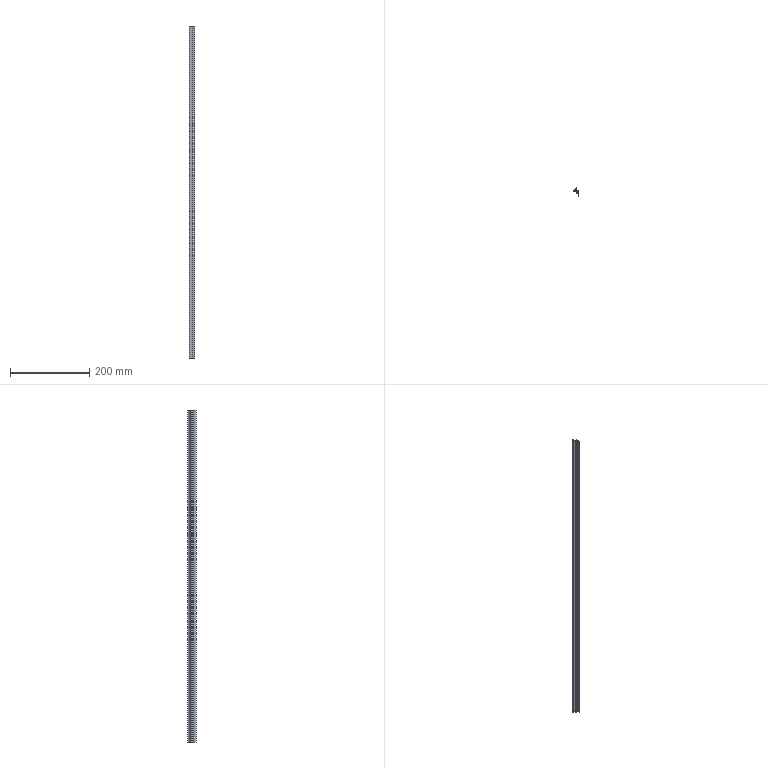Part | SolidWorks | features BaseBody 1, ICE 1, MoveFace 1 | 1 solid | 27 faces | box 14 x 20.3 x 840 mm | volume 42769 mm3 | plane 20 | cylinder 7 | commonest cylinder face diameters 0.387 x2 0.8 x2 0.4 x1 20 x1 22 x1
STEP:
#1=CARTESIAN_POINT('',(-5.304,-0.625,200.));
#2=VERTEX_POINT('',#1);
#3=CARTESIAN_POINT('',(-5.449,-0.8125,200.));
#4=VERTEX_POINT('',#3);
#5=CARTESIAN_POINT('',(-5.255,-0.8125,200.));
#6=DIRECTION('',(0.,0.,1.));
#7=DIRECTION('',(-1.,0.,0.));
#8=AXIS2_PLACEMENT_3D('',#5,#6,#7);
#9=CIRCLE('',#8,0.1937);
#10=EDGE_CURVE('',#2,#4,#9,.T.);
#11=ORIENTED_EDGE('',*,*,#10,.T.);
#12=CARTESIAN_POINT('',(-5.449,-0.8125,-640.));
#13=VERTEX_POINT('',#12);
#14=CARTESIAN_POINT('',(-5.449,-0.8125,230.));
#15=DIRECTION('',(0.,0.,-1.));
#16=VECTOR('',#15,1000.);
#17=LINE('',#14,#16);
#18=EDGE_CURVE('',#4,#13,#17,.T.);
#19=ORIENTED_EDGE('',*,*,#18,.T.);
#20=CARTESIAN_POINT('',(-5.304,-0.625,-640.));
#21=VERTEX_POINT('',#20);
#22=CARTESIAN_POINT('',(-5.255,-0.8125,-640.));
#23=DIRECTION('',(0.,0.,-1.));
#24=DIRECTION('',(1.,0.,0.));
#25=AXIS2_PLACEMENT_3D('',#22,#23,#24);
#26=CIRCLE('',#25,0.1937);
#27=EDGE_CURVE('',#13,#21,#26,.T.);
#28=ORIENTED_EDGE('',*,*,#27,.T.);
#29=CARTESIAN_POINT('',(-5.304,-0.625,230.));
#30=DIRECTION('',(0.,0.,-1.));
#31=VECTOR('',#30,1000.);
#32=LINE('',#29,#31);
#33=EDGE_CURVE('',#2,#21,#32,.T.);
#34=ORIENTED_EDGE('',*,*,#33,.F.);
#35=EDGE_LOOP('',(#11,#19,#28,#34));
#36=FACE_OUTER_BOUND('',#35,.T.);
#37=CARTESIAN_POINT('',(-5.255,-0.8125,230.));
#38=DIRECTION('',(0.,0.,-1.));
#39=DIRECTION('',(-1.,0.,0.));
#40=AXIS2_PLACEMENT_3D('',#37,#38,#39);
#41=CYLINDRICAL_SURFACE('',#40,0.1937);
#42=ADVANCED_FACE('',(#36),#41,.F.);
#43=CARTESIAN_POINT('',(5.,-1.,-640.));
#44=VERTEX_POINT('',#43);
#45=CARTESIAN_POINT('',(5.,-14.3,-640.));
#46=VERTEX_POINT('',#45);
#47=CARTESIAN_POINT('',(5.,29.623,-640.));
#48=DIRECTION('',(0.,-1.,0.));
#49=VECTOR('',#48,1000.);
#50=LINE('',#47,#49);
#51=EDGE_CURVE('',#44,#46,#50,.T.);
#52=ORIENTED_EDGE('',*,*,#51,.F.);
#53=CARTESIAN_POINT('',(5.,-1.,200.));
#54=VERTEX_POINT('',#53);
#55=CARTESIAN_POINT('',(5.,-1.,230.));
#56=DIRECTION('',(0.,0.,-1.));
#57=VECTOR('',#56,1000.);
#58=LINE('',#55,#57);
#59=EDGE_CURVE('',#54,#44,#58,.T.);
#60=ORIENTED_EDGE('',*,*,#59,.F.);
#61=CARTESIAN_POINT('',(5.,-14.3,200.));
#62=VERTEX_POINT('',#61);
#63=CARTESIAN_POINT('',(5.,-14.3,200.));
#64=DIRECTION('',(0.,1.,0.));
#65=VECTOR('',#64,1000.);
#66=LINE('',#63,#65);
#67=EDGE_CURVE('',#62,#54,#66,.T.);
#68=ORIENTED_EDGE('',*,*,#67,.F.);
#69=CARTESIAN_POINT('',(5.,-14.3,230.));
#70=DIRECTION('',(0.,0.,1.));
#71=VECTOR('',#70,1000.);
#72=LINE('',#69,#71);
#73=EDGE_CURVE('',#46,#62,#72,.T.);
#74=ORIENTED_EDGE('',*,*,#73,.F.);
#75=EDGE_LOOP('',(#52,#60,#68,#74));
#76=FACE_OUTER_BOUND('',#75,.T.);
#77=CARTESIAN_POINT('',(5.,-14.3,230.));
#78=DIRECTION('',(-1.,0.,0.));
#79=DIRECTION('',(0.,0.,1.));
#80=AXIS2_PLACEMENT_3D('',#77,#78,#79);
#81=PLANE('',#80);
#82=ADVANCED_FACE('',(#76),#81,.F.);
#83=CARTESIAN_POINT('',(-9.,-2.,-640.));
#84=VERTEX_POINT('',#83);
#85=CARTESIAN_POINT('',(-9.,-2.,200.));
#86=VERTEX_POINT('',#85);
#87=CARTESIAN_POINT('',(-9.,-2.,230.));
#88=DIRECTION('',(0.,0.,1.));
#89=VECTOR('',#88,1000.);
#90=LINE('',#87,#89);
#91=EDGE_CURVE('',#84,#86,#90,.T.);
#92=ORIENTED_EDGE('',*,*,#91,.F.);
#93=CARTESIAN_POINT('',(0.9,-2.,-640.));
#94=VERTEX_POINT('',#93);
#95=CARTESIAN_POINT('',(5.,-2.,-640.));
#96=DIRECTION('',(-1.,0.,0.));
#97=VECTOR('',#96,1000.);
#98=LINE('',#95,#97);
#99=EDGE_CURVE('',#94,#84,#98,.T.);
#100=ORIENTED_EDGE('',*,*,#99,.F.);
#101=CARTESIAN_POINT('',(0.9,-2.,200.));
#102=VERTEX_POINT('',#101);
#103=CARTESIAN_POINT('',(0.9,-2.,230.));
#104=DIRECTION('',(0.,0.,-1.));
#105=VECTOR('',#104,1000.);
#106=LINE('',#103,#105);
#107=EDGE_CURVE('',#102,#94,#106,.T.);
#108=ORIENTED_EDGE('',*,*,#107,.F.);
#109=CARTESIAN_POINT('',(5.,-2.,200.));
#110=DIRECTION('',(1.,0.,0.));
#111=VECTOR('',#110,1000.);
#112=LINE('',#109,#111);
#113=EDGE_CURVE('',#86,#102,#112,.T.);
#114=ORIENTED_EDGE('',*,*,#113,.F.);
#115=EDGE_LOOP('',(#92,#100,#108,#114));
#116=FACE_OUTER_BOUND('',#115,.T.);
#117=CARTESIAN_POINT('',(-9.,-2.,230.));
#118=DIRECTION('',(0.,1.,0.));
#119=DIRECTION('',(0.,0.,1.));
#120=AXIS2_PLACEMENT_3D('',#117,#118,#119);
#121=PLANE('',#120);
#122=ADVANCED_FACE('',(#116),#121,.F.);
#123=CARTESIAN_POINT('',(4.,-6.,200.));
#124=VERTEX_POINT('',#123);
#125=CARTESIAN_POINT('',(4.,-3.,200.));
#126=VERTEX_POINT('',#125);
#127=CARTESIAN_POINT('',(4.,29.623,200.));
#128=DIRECTION('',(0.,1.,0.));
#129=VECTOR('',#128,1000.);
#130=LINE('',#127,#129);
#131=EDGE_CURVE('',#124,#126,#130,.T.);
#132=ORIENTED_EDGE('',*,*,#131,.F.);
#133=CARTESIAN_POINT('',(1.,-6.,200.));
#134=VERTEX_POINT('',#133);
#135=CARTESIAN_POINT('',(5.,-6.,200.));
#136=DIRECTION('',(1.,0.,0.));
#137=VECTOR('',#136,1000.);
#138=LINE('',#135,#137);
#139=EDGE_CURVE('',#134,#124,#138,.T.);
#140=ORIENTED_EDGE('',*,*,#139,.F.);
#141=CARTESIAN_POINT('',(1.,-6.7,200.));
#142=VERTEX_POINT('',#141);
#143=CARTESIAN_POINT('',(1.,-6.,200.));
#144=DIRECTION('',(0.,-1.,0.));
#145=VECTOR('',#144,1000.);
#146=LINE('',#143,#145);
#147=EDGE_CURVE('',#134,#142,#146,.T.);
#148=ORIENTED_EDGE('',*,*,#147,.T.);
#149=CARTESIAN_POINT('',(-1.7,-6.7,200.));
#150=VERTEX_POINT('',#149);
#151=CARTESIAN_POINT('',(5.,-6.7,200.));
#152=DIRECTION('',(1.,0.,0.));
#153=VECTOR('',#152,1000.);
#154=LINE('',#151,#153);
#155=EDGE_CURVE('',#150,#142,#154,.T.);
#156=ORIENTED_EDGE('',*,*,#155,.F.);
#157=CARTESIAN_POINT('',(-1.7,-7.7,200.));
#158=VERTEX_POINT('',#157);
#159=CARTESIAN_POINT('',(-1.7,-6.7,200.));
#160=DIRECTION('',(0.,-1.,0.));
#161=VECTOR('',#160,1000.);
#162=LINE('',#159,#161);
#163=EDGE_CURVE('',#150,#158,#162,.T.);
#164=ORIENTED_EDGE('',*,*,#163,.T.);
#165=CARTESIAN_POINT('',(4.,-7.7,200.));
#166=VERTEX_POINT('',#165);
#167=CARTESIAN_POINT('',(5.,-7.7,200.));
#168=DIRECTION('',(-1.,0.,0.));
#169=VECTOR('',#168,1000.);
#170=LINE('',#167,#169);
#171=EDGE_CURVE('',#166,#158,#170,.T.);
#172=ORIENTED_EDGE('',*,*,#171,.F.);
#173=CARTESIAN_POINT('',(4.,-14.3,200.));
#174=VERTEX_POINT('',#173);
#175=CARTESIAN_POINT('',(4.,29.623,200.));
#176=DIRECTION('',(0.,1.,0.));
#177=VECTOR('',#176,1000.);
#178=LINE('',#175,#177);
#179=EDGE_CURVE('',#174,#166,#178,.T.);
#180=ORIENTED_EDGE('',*,*,#179,.F.);
#181=CARTESIAN_POINT('',(5.,-14.3,200.));
#182=DIRECTION('',(-1.,0.,0.));
#183=VECTOR('',#182,1000.);
#184=LINE('',#181,#183);
#185=EDGE_CURVE('',#62,#174,#184,.T.);
#186=ORIENTED_EDGE('',*,*,#185,.F.);
#187=ORIENTED_EDGE('',*,*,#67,.T.);
#188=CARTESIAN_POINT('',(-5.207,-1.,200.));
#189=VERTEX_POINT('',#188);
#190=CARTESIAN_POINT('',(5.,-1.,200.));
#191=DIRECTION('',(1.,0.,0.));
#192=VECTOR('',#191,1000.);
#193=LINE('',#190,#192);
#194=EDGE_CURVE('',#189,#54,#193,.T.);
#195=ORIENTED_EDGE('',*,*,#194,.F.);
#196=CARTESIAN_POINT('',(-5.255,-0.8125,200.));
#197=DIRECTION('',(0.,0.,1.));
#198=DIRECTION('',(-1.,0.,0.));
#199=AXIS2_PLACEMENT_3D('',#196,#197,#198);
#200=CIRCLE('',#199,0.1937);
#201=EDGE_CURVE('',#4,#189,#200,.T.);
#202=ORIENTED_EDGE('',*,*,#201,.F.);
#203=ORIENTED_EDGE('',*,*,#10,.F.);
#204=CARTESIAN_POINT('',(-1.368,3.063,200.));
#205=VERTEX_POINT('',#204);
#206=CARTESIAN_POINT('',(-10.628,9.,200.));
#207=DIRECTION('',(0.,0.,1.));
#208=DIRECTION('',(-1.,0.,0.));
#209=AXIS2_PLACEMENT_3D('',#206,#207,#208);
#210=CIRCLE('',#209,11.);
#211=EDGE_CURVE('',#2,#205,#210,.T.);
#212=ORIENTED_EDGE('',*,*,#211,.T.);
#213=CARTESIAN_POINT('',(-1.,2.955,200.));
#214=VERTEX_POINT('',#213);
#215=CARTESIAN_POINT('',(-1.2,2.955,200.));
#216=DIRECTION('',(0.,0.,1.));
#217=DIRECTION('',(-1.,0.,0.));
#218=AXIS2_PLACEMENT_3D('',#215,#216,#217);
#219=CIRCLE('',#218,0.2);
#220=EDGE_CURVE('',#214,#205,#219,.T.);
#221=ORIENTED_EDGE('',*,*,#220,.F.);
#222=CARTESIAN_POINT('',(-1.,1.5,200.));
#223=VERTEX_POINT('',#222);
#224=CARTESIAN_POINT('',(-1.,2.955,200.));
#225=DIRECTION('',(0.,1.,0.));
#226=VECTOR('',#225,1000.);
#227=LINE('',#224,#226);
#228=EDGE_CURVE('',#223,#214,#227,.T.);
#229=ORIENTED_EDGE('',*,*,#228,.F.);
#230=CARTESIAN_POINT('',(0.,1.5,200.));
#231=VERTEX_POINT('',#230);
#232=CARTESIAN_POINT('',(-1.,1.5,200.));
#233=DIRECTION('',(-1.,0.,0.));
#234=VECTOR('',#233,1000.);
#235=LINE('',#232,#234);
#236=EDGE_CURVE('',#231,#223,#235,.T.);
#237=ORIENTED_EDGE('',*,*,#236,.F.);
#238=CARTESIAN_POINT('',(0.,6.,200.));
#239=VERTEX_POINT('',#238);
#240=CARTESIAN_POINT('',(0.,1.5,200.));
#241=DIRECTION('',(0.,-1.,0.));
#242=VECTOR('',#241,1000.);
#243=LINE('',#240,#242);
#244=EDGE_CURVE('',#239,#231,#243,.T.);
#245=ORIENTED_EDGE('',*,*,#244,.F.);
#246=CARTESIAN_POINT('',(-0.8,6.,200.));
#247=VERTEX_POINT('',#246);
#248=CARTESIAN_POINT('',(0.,6.,200.));
#249=DIRECTION('',(1.,0.,0.));
#250=VECTOR('',#249,1000.);
#251=LINE('',#248,#250);
#252=EDGE_CURVE('',#247,#239,#251,.T.);
#253=ORIENTED_EDGE('',*,*,#252,.F.);
#254=CARTESIAN_POINT('',(-1.178,5.731,200.));
#255=VERTEX_POINT('',#254);
#256=CARTESIAN_POINT('',(-0.8,5.6,200.));
#257=DIRECTION('',(0.,0.,1.));
#258=DIRECTION('',(-1.,0.,0.));
#259=AXIS2_PLACEMENT_3D('',#256,#257,#258);
#260=CIRCLE('',#259,0.4);
#261=EDGE_CURVE('',#247,#255,#260,.T.);
#262=ORIENTED_EDGE('',*,*,#261,.T.);
#263=CARTESIAN_POINT('',(-8.678,-0.8077,200.));
#264=VERTEX_POINT('',#263);
#265=CARTESIAN_POINT('',(-10.628,9.,200.));
#266=DIRECTION('',(0.,0.,1.));
#267=DIRECTION('',(-1.,0.,0.));
#268=AXIS2_PLACEMENT_3D('',#265,#266,#267);
#269=CIRCLE('',#268,10.);
#270=EDGE_CURVE('',#264,#255,#269,.T.);
#271=ORIENTED_EDGE('',*,*,#270,.F.);
#272=CARTESIAN_POINT('',(-9.,-1.2,200.));
#273=VERTEX_POINT('',#272);
#274=CARTESIAN_POINT('',(-8.6,-1.2,200.));
#275=DIRECTION('',(0.,0.,1.));
#276=DIRECTION('',(-1.,0.,0.));
#277=AXIS2_PLACEMENT_3D('',#274,#275,#276);
#278=CIRCLE('',#277,0.4);
#279=EDGE_CURVE('',#264,#273,#278,.T.);
#280=ORIENTED_EDGE('',*,*,#279,.T.);
#281=CARTESIAN_POINT('',(-9.,8.,200.));
#282=DIRECTION('',(0.,-1.,0.));
#283=VECTOR('',#282,1000.);
#284=LINE('',#281,#283);
#285=EDGE_CURVE('',#273,#86,#284,.T.);
#286=ORIENTED_EDGE('',*,*,#285,.T.);
#287=ORIENTED_EDGE('',*,*,#113,.T.);
#288=CARTESIAN_POINT('',(0.9,-3.,200.));
#289=VERTEX_POINT('',#288);
#290=CARTESIAN_POINT('',(0.9,29.623,200.));
#291=DIRECTION('',(0.,1.,0.));
#292=VECTOR('',#291,1000.);
#293=LINE('',#290,#292);
#294=EDGE_CURVE('',#289,#102,#293,.T.);
#295=ORIENTED_EDGE('',*,*,#294,.F.);
#296=CARTESIAN_POINT('',(5.,-3.,200.));
#297=DIRECTION('',(-1.,0.,0.));
#298=VECTOR('',#297,1000.);
#299=LINE('',#296,#298);
#300=EDGE_CURVE('',#126,#289,#299,.T.);
#301=ORIENTED_EDGE('',*,*,#300,.F.);
#302=EDGE_LOOP('',(#132,#140,#148,#156,#164,#172,#180,#186,#187,#195,#202,#203,#212,#221,#229,#237,#245,#253,#262,#271,#280,#286,#287,#295,#301));
#303=FACE_OUTER_BOUND('',#302,.T.);
#304=CARTESIAN_POINT('',(5.,29.623,200.));
#305=DIRECTION('',(0.,0.,-1.));
#306=DIRECTION('',(-1.,0.,0.));
#307=AXIS2_PLACEMENT_3D('',#304,#305,#306);
#308=PLANE('',#307);
#309=ADVANCED_FACE('',(#303),#308,.F.);
#310=ORIENTED_EDGE('',*,*,#185,.T.);
#311=CARTESIAN_POINT('',(4.,-14.3,-640.));
#312=VERTEX_POINT('',#311);
#313=CARTESIAN_POINT('',(4.,-14.3,230.));
#314=DIRECTION('',(0.,0.,1.));
#315=VECTOR('',#314,1000.);
#316=LINE('',#313,#315);
#317=EDGE_CURVE('',#312,#174,#316,.T.);
#318=ORIENTED_EDGE('',*,*,#317,.F.);
#319=CARTESIAN_POINT('',(5.,-14.3,-640.));
#320=DIRECTION('',(-1.,0.,0.));
#321=VECTOR('',#320,1000.);
#322=LINE('',#319,#321);
#323=EDGE_CURVE('',#46,#312,#322,.T.);
#324=ORIENTED_EDGE('',*,*,#323,.F.);
#325=ORIENTED_EDGE('',*,*,#73,.T.);
#326=EDGE_LOOP('',(#310,#318,#324,#325));
#327=FACE_OUTER_BOUND('',#326,.T.);
#328=CARTESIAN_POINT('',(4.,-14.3,230.));
#329=DIRECTION('',(0.,1.,0.));
#330=DIRECTION('',(0.,0.,1.));
#331=AXIS2_PLACEMENT_3D('',#328,#329,#330);
#332=PLANE('',#331);
#333=ADVANCED_FACE('',(#327),#332,.F.);
#334=ORIENTED_EDGE('',*,*,#51,.T.);
#335=ORIENTED_EDGE('',*,*,#323,.T.);
#336=CARTESIAN_POINT('',(4.,-7.7,-640.));
#337=VERTEX_POINT('',#336);
#338=CARTESIAN_POINT('',(4.,-7.7,-640.));
#339=DIRECTION('',(0.,-1.,0.));
#340=VECTOR('',#339,1000.);
#341=LINE('',#338,#340);
#342=EDGE_CURVE('',#337,#312,#341,.T.);
#343=ORIENTED_EDGE('',*,*,#342,.F.);
#344=CARTESIAN_POINT('',(-1.7,-7.7,-640.));
#345=VERTEX_POINT('',#344);
#346=CARTESIAN_POINT('',(-1.7,-7.7,-640.));
#347=DIRECTION('',(1.,0.,0.));
#348=VECTOR('',#347,1000.);
#349=LINE('',#346,#348);
#350=EDGE_CURVE('',#345,#337,#349,.T.);
#351=ORIENTED_EDGE('',*,*,#350,.F.);
#352=CARTESIAN_POINT('',(-1.7,-6.7,-640.));
#353=VERTEX_POINT('',#352);
#354=CARTESIAN_POINT('',(-1.7,29.623,-640.));
#355=DIRECTION('',(0.,1.,0.));
#356=VECTOR('',#355,1000.);
#357=LINE('',#354,#356);
#358=EDGE_CURVE('',#345,#353,#357,.T.);
#359=ORIENTED_EDGE('',*,*,#358,.T.);
#360=CARTESIAN_POINT('',(1.,-6.7,-640.));
#361=VERTEX_POINT('',#360);
#362=CARTESIAN_POINT('',(1.,-6.7,-640.));
#363=DIRECTION('',(-1.,0.,0.));
#364=VECTOR('',#363,1000.);
#365=LINE('',#362,#364);
#366=EDGE_CURVE('',#361,#353,#365,.T.);
#367=ORIENTED_EDGE('',*,*,#366,.F.);
#368=CARTESIAN_POINT('',(1.,-6.,-640.));
#369=VERTEX_POINT('',#368);
#370=CARTESIAN_POINT('',(1.,29.623,-640.));
#371=DIRECTION('',(0.,1.,0.));
#372=VECTOR('',#371,1000.);
#373=LINE('',#370,#372);
#374=EDGE_CURVE('',#361,#369,#373,.T.);
#375=ORIENTED_EDGE('',*,*,#374,.T.);
#376=CARTESIAN_POINT('',(4.,-6.,-640.));
#377=VERTEX_POINT('',#376);
#378=CARTESIAN_POINT('',(4.,-6.,-640.));
#379=DIRECTION('',(-1.,0.,0.));
#380=VECTOR('',#379,1000.);
#381=LINE('',#378,#380);
#382=EDGE_CURVE('',#377,#369,#381,.T.);
#383=ORIENTED_EDGE('',*,*,#382,.F.);
#384=CARTESIAN_POINT('',(4.,-3.,-640.));
#385=VERTEX_POINT('',#384);
#386=CARTESIAN_POINT('',(4.,-3.,-640.));
#387=DIRECTION('',(0.,-1.,0.));
#388=VECTOR('',#387,1000.);
#389=LINE('',#386,#388);
#390=EDGE_CURVE('',#385,#377,#389,.T.);
#391=ORIENTED_EDGE('',*,*,#390,.F.);
#392=CARTESIAN_POINT('',(0.9,-3.,-640.));
#393=VERTEX_POINT('',#392);
#394=CARTESIAN_POINT('',(0.9,-3.,-640.));
#395=DIRECTION('',(1.,0.,0.));
#396=VECTOR('',#395,1000.);
#397=LINE('',#394,#396);
#398=EDGE_CURVE('',#393,#385,#397,.T.);
#399=ORIENTED_EDGE('',*,*,#398,.F.);
#400=CARTESIAN_POINT('',(0.9,-2.,-640.));
#401=DIRECTION('',(0.,-1.,0.));
#402=VECTOR('',#401,1000.);
#403=LINE('',#400,#402);
#404=EDGE_CURVE('',#94,#393,#403,.T.);
#405=ORIENTED_EDGE('',*,*,#404,.F.);
#406=ORIENTED_EDGE('',*,*,#99,.T.);
#407=CARTESIAN_POINT('',(-9.,-1.2,-640.));
#408=VERTEX_POINT('',#407);
#409=CARTESIAN_POINT('',(-9.,-1.2,-640.));
#410=DIRECTION('',(0.,-1.,0.));
#411=VECTOR('',#410,1000.);
#412=LINE('',#409,#411);
#413=EDGE_CURVE('',#408,#84,#412,.T.);
#414=ORIENTED_EDGE('',*,*,#413,.F.);
#415=CARTESIAN_POINT('',(-8.678,-0.8077,-640.));
#416=VERTEX_POINT('',#415);
#417=CARTESIAN_POINT('',(-8.6,-1.2,-640.));
#418=DIRECTION('',(0.,0.,-1.));
#419=DIRECTION('',(1.,0.,0.));
#420=AXIS2_PLACEMENT_3D('',#417,#418,#419);
#421=CIRCLE('',#420,0.4);
#422=EDGE_CURVE('',#408,#416,#421,.T.);
#423=ORIENTED_EDGE('',*,*,#422,.T.);
#424=CARTESIAN_POINT('',(-1.178,5.731,-640.));
#425=VERTEX_POINT('',#424);
#426=CARTESIAN_POINT('',(-10.628,9.,-640.));
#427=DIRECTION('',(0.,0.,-1.));
#428=DIRECTION('',(1.,0.,0.));
#429=AXIS2_PLACEMENT_3D('',#426,#427,#428);
#430=CIRCLE('',#429,10.);
#431=EDGE_CURVE('',#425,#416,#430,.T.);
#432=ORIENTED_EDGE('',*,*,#431,.F.);
#433=CARTESIAN_POINT('',(-0.8,6.,-640.));
#434=VERTEX_POINT('',#433);
#435=CARTESIAN_POINT('',(-0.8,5.6,-640.));
#436=DIRECTION('',(0.,0.,-1.));
#437=DIRECTION('',(1.,0.,0.));
#438=AXIS2_PLACEMENT_3D('',#435,#436,#437);
#439=CIRCLE('',#438,0.4);
#440=EDGE_CURVE('',#425,#434,#439,.T.);
#441=ORIENTED_EDGE('',*,*,#440,.T.);
#442=CARTESIAN_POINT('',(0.,6.,-640.));
#443=VERTEX_POINT('',#442);
#444=CARTESIAN_POINT('',(0.,6.,-640.));
#445=DIRECTION('',(-1.,0.,0.));
#446=VECTOR('',#445,1000.);
#447=LINE('',#444,#446);
#448=EDGE_CURVE('',#443,#434,#447,.T.);
#449=ORIENTED_EDGE('',*,*,#448,.F.);
#450=CARTESIAN_POINT('',(0.,1.5,-640.));
#451=VERTEX_POINT('',#450);
#452=CARTESIAN_POINT('',(0.,1.5,-640.));
#453=DIRECTION('',(0.,1.,0.));
#454=VECTOR('',#453,1000.);
#455=LINE('',#452,#454);
#456=EDGE_CURVE('',#451,#443,#455,.T.);
#457=ORIENTED_EDGE('',*,*,#456,.F.);
#458=CARTESIAN_POINT('',(-1.,1.5,-640.));
#459=VERTEX_POINT('',#458);
#460=CARTESIAN_POINT('',(-1.,1.5,-640.));
#461=DIRECTION('',(1.,0.,0.));
#462=VECTOR('',#461,1000.);
#463=LINE('',#460,#462);
#464=EDGE_CURVE('',#459,#451,#463,.T.);
#465=ORIENTED_EDGE('',*,*,#464,.F.);
#466=CARTESIAN_POINT('',(-1.,2.955,-640.));
#467=VERTEX_POINT('',#466);
#468=CARTESIAN_POINT('',(-1.,2.955,-640.));
#469=DIRECTION('',(0.,-1.,0.));
#470=VECTOR('',#469,1000.);
#471=LINE('',#468,#470);
#472=EDGE_CURVE('',#467,#459,#471,.T.);
#473=ORIENTED_EDGE('',*,*,#472,.F.);
#474=CARTESIAN_POINT('',(-1.368,3.063,-640.));
#475=VERTEX_POINT('',#474);
#476=CARTESIAN_POINT('',(-1.2,2.955,-640.));
#477=DIRECTION('',(0.,0.,-1.));
#478=DIRECTION('',(1.,0.,0.));
#479=AXIS2_PLACEMENT_3D('',#476,#477,#478);
#480=CIRCLE('',#479,0.2);
#481=EDGE_CURVE('',#475,#467,#480,.T.);
#482=ORIENTED_EDGE('',*,*,#481,.F.);
#483=CARTESIAN_POINT('',(-10.628,9.,-640.));
#484=DIRECTION('',(0.,0.,-1.));
#485=DIRECTION('',(1.,0.,0.));
#486=AXIS2_PLACEMENT_3D('',#483,#484,#485);
#487=CIRCLE('',#486,11.);
#488=EDGE_CURVE('',#475,#21,#487,.T.);
#489=ORIENTED_EDGE('',*,*,#488,.T.);
#490=ORIENTED_EDGE('',*,*,#27,.F.);
#491=CARTESIAN_POINT('',(-5.207,-1.,-640.));
#492=VERTEX_POINT('',#491);
#493=CARTESIAN_POINT('',(-5.255,-0.8125,-640.));
#494=DIRECTION('',(0.,0.,-1.));
#495=DIRECTION('',(1.,0.,0.));
#496=AXIS2_PLACEMENT_3D('',#493,#494,#495);
#497=CIRCLE('',#496,0.1937);
#498=EDGE_CURVE('',#492,#13,#497,.T.);
#499=ORIENTED_EDGE('',*,*,#498,.F.);
#500=CARTESIAN_POINT('',(5.,-1.,-640.));
#501=DIRECTION('',(-1.,0.,0.));
#502=VECTOR('',#501,1000.);
#503=LINE('',#500,#502);
#504=EDGE_CURVE('',#44,#492,#503,.T.);
#505=ORIENTED_EDGE('',*,*,#504,.F.);
#506=EDGE_LOOP('',(#334,#335,#343,#351,#359,#367,#375,#383,#391,#399,#405,#406,#414,#423,#432,#441,#449,#457,#465,#473,#482,#489,#490,#499,#505));
#507=FACE_OUTER_BOUND('',#506,.T.);
#508=CARTESIAN_POINT('',(5.,29.623,-640.));
#509=DIRECTION('',(0.,0.,1.));
#510=DIRECTION('',(1.,0.,0.));
#511=AXIS2_PLACEMENT_3D('',#508,#509,#510);
#512=PLANE('',#511);
#513=ADVANCED_FACE('',(#507),#512,.F.);
#514=ORIENTED_EDGE('',*,*,#59,.T.);
#515=ORIENTED_EDGE('',*,*,#504,.T.);
#516=CARTESIAN_POINT('',(-5.207,-1.,230.));
#517=DIRECTION('',(0.,0.,-1.));
#518=VECTOR('',#517,1000.);
#519=LINE('',#516,#518);
#520=EDGE_CURVE('',#189,#492,#519,.T.);
#521=ORIENTED_EDGE('',*,*,#520,.F.);
#522=ORIENTED_EDGE('',*,*,#194,.T.);
#523=EDGE_LOOP('',(#514,#515,#521,#522));
#524=FACE_OUTER_BOUND('',#523,.T.);
#525=CARTESIAN_POINT('',(5.,-1.,230.));
#526=DIRECTION('',(0.,-1.,0.));
#527=DIRECTION('',(0.,0.,-1.));
#528=AXIS2_PLACEMENT_3D('',#525,#526,#527);
#529=PLANE('',#528);
#530=ADVANCED_FACE('',(#524),#529,.F.);
#531=CARTESIAN_POINT('',(-9.,-1.2,230.));
#532=DIRECTION('',(0.,0.,1.));
#533=VECTOR('',#532,1000.);
#534=LINE('',#531,#533);
#535=EDGE_CURVE('',#408,#273,#534,.T.);
#536=ORIENTED_EDGE('',*,*,#535,.F.);
#537=ORIENTED_EDGE('',*,*,#413,.T.);
#538=ORIENTED_EDGE('',*,*,#91,.T.);
#539=ORIENTED_EDGE('',*,*,#285,.F.);
#540=EDGE_LOOP('',(#536,#537,#538,#539));
#541=FACE_OUTER_BOUND('',#540,.T.);
#542=CARTESIAN_POINT('',(-9.,-1.2,230.));
#543=DIRECTION('',(1.,0.,0.));
#544=DIRECTION('',(0.,0.,-1.));
#545=AXIS2_PLACEMENT_3D('',#542,#543,#544);
#546=PLANE('',#545);
#547=ADVANCED_FACE('',(#541),#546,.F.);
#548=ORIENTED_EDGE('',*,*,#294,.T.);
#549=ORIENTED_EDGE('',*,*,#107,.T.);
#550=ORIENTED_EDGE('',*,*,#404,.T.);
#551=CARTESIAN_POINT('',(0.9,-3.,230.));
#552=DIRECTION('',(0.,0.,-1.));
#553=VECTOR('',#552,1000.);
#554=LINE('',#551,#553);
#555=EDGE_CURVE('',#289,#393,#554,.T.);
#556=ORIENTED_EDGE('',*,*,#555,.F.);
#557=EDGE_LOOP('',(#548,#549,#550,#556));
#558=FACE_OUTER_BOUND('',#557,.T.);
#559=CARTESIAN_POINT('',(0.9,-2.,230.));
#560=DIRECTION('',(1.,0.,0.));
#561=DIRECTION('',(0.,0.,-1.));
#562=AXIS2_PLACEMENT_3D('',#559,#560,#561);
#563=PLANE('',#562);
#564=ADVANCED_FACE('',(#558),#563,.F.);
#565=ORIENTED_EDGE('',*,*,#300,.T.);
#566=ORIENTED_EDGE('',*,*,#555,.T.);
#567=ORIENTED_EDGE('',*,*,#398,.T.);
#568=CARTESIAN_POINT('',(4.,-3.,230.));
#569=DIRECTION('',(0.,0.,-1.));
#570=VECTOR('',#569,1000.);
#571=LINE('',#568,#570);
#572=EDGE_CURVE('',#126,#385,#571,.T.);
#573=ORIENTED_EDGE('',*,*,#572,.F.);
#574=EDGE_LOOP('',(#565,#566,#567,#573));
#575=FACE_OUTER_BOUND('',#574,.T.);
#576=CARTESIAN_POINT('',(0.9,-3.,230.));
#577=DIRECTION('',(0.,1.,0.));
#578=DIRECTION('',(0.,0.,1.));
#579=AXIS2_PLACEMENT_3D('',#576,#577,#578);
#580=PLANE('',#579);
#581=ADVANCED_FACE('',(#575),#580,.F.);
#582=ORIENTED_EDGE('',*,*,#131,.T.);
#583=ORIENTED_EDGE('',*,*,#572,.T.);
#584=ORIENTED_EDGE('',*,*,#390,.T.);
#585=CARTESIAN_POINT('',(4.,-6.,230.));
#586=DIRECTION('',(0.,0.,-1.));
#587=VECTOR('',#586,1000.);
#588=LINE('',#585,#587);
#589=EDGE_CURVE('',#124,#377,#588,.T.);
#590=ORIENTED_EDGE('',*,*,#589,.F.);
#591=EDGE_LOOP('',(#582,#583,#584,#590));
#592=FACE_OUTER_BOUND('',#591,.T.);
#593=CARTESIAN_POINT('',(4.,-3.,230.));
#594=DIRECTION('',(1.,0.,0.));
#595=DIRECTION('',(0.,0.,-1.));
#596=AXIS2_PLACEMENT_3D('',#593,#594,#595);
#597=PLANE('',#596);
#598=ADVANCED_FACE('',(#592),#597,.F.);
#599=ORIENTED_EDGE('',*,*,#139,.T.);
#600=ORIENTED_EDGE('',*,*,#589,.T.);
#601=ORIENTED_EDGE('',*,*,#382,.T.);
#602=CARTESIAN_POINT('',(1.,-6.,230.));
#603=DIRECTION('',(0.,0.,-1.));
#604=VECTOR('',#603,1000.);
#605=LINE('',#602,#604);
#606=EDGE_CURVE('',#134,#369,#605,.T.);
#607=ORIENTED_EDGE('',*,*,#606,.F.);
#608=EDGE_LOOP('',(#599,#600,#601,#607));
#609=FACE_OUTER_BOUND('',#608,.T.);
#610=CARTESIAN_POINT('',(4.,-6.,230.));
#611=DIRECTION('',(0.,-1.,0.));
#612=DIRECTION('',(0.,0.,-1.));
#613=AXIS2_PLACEMENT_3D('',#610,#611,#612);
#614=PLANE('',#613);
#615=ADVANCED_FACE('',(#609),#614,.F.);
#616=ORIENTED_EDGE('',*,*,#155,.T.);
#617=CARTESIAN_POINT('',(1.,-6.7,230.));
#618=DIRECTION('',(0.,0.,1.));
#619=VECTOR('',#618,1000.);
#620=LINE('',#617,#619);
#621=EDGE_CURVE('',#361,#142,#620,.T.);
#622=ORIENTED_EDGE('',*,*,#621,.F.);
#623=ORIENTED_EDGE('',*,*,#366,.T.);
#624=CARTESIAN_POINT('',(-1.7,-6.7,230.));
#625=DIRECTION('',(0.,0.,-1.));
#626=VECTOR('',#625,1000.);
#627=LINE('',#624,#626);
#628=EDGE_CURVE('',#150,#353,#627,.T.);
#629=ORIENTED_EDGE('',*,*,#628,.F.);
#630=EDGE_LOOP('',(#616,#622,#623,#629));
#631=FACE_OUTER_BOUND('',#630,.T.);
#632=CARTESIAN_POINT('',(1.,-6.7,230.));
#633=DIRECTION('',(0.,-1.,0.));
#634=DIRECTION('',(0.,0.,-1.));
#635=AXIS2_PLACEMENT_3D('',#632,#633,#634);
#636=PLANE('',#635);
#637=ADVANCED_FACE('',(#631),#636,.F.);
#638=ORIENTED_EDGE('',*,*,#171,.T.);
#639=CARTESIAN_POINT('',(-1.7,-7.7,230.));
#640=DIRECTION('',(0.,0.,1.));
#641=VECTOR('',#640,1000.);
#642=LINE('',#639,#641);
#643=EDGE_CURVE('',#345,#158,#642,.T.);
#644=ORIENTED_EDGE('',*,*,#643,.F.);
#645=ORIENTED_EDGE('',*,*,#350,.T.);
#646=CARTESIAN_POINT('',(4.,-7.7,230.));
#647=DIRECTION('',(0.,0.,-1.));
#648=VECTOR('',#647,1000.);
#649=LINE('',#646,#648);
#650=EDGE_CURVE('',#166,#337,#649,.T.);
#651=ORIENTED_EDGE('',*,*,#650,.F.);
#652=EDGE_LOOP('',(#638,#644,#645,#651));
#653=FACE_OUTER_BOUND('',#652,.T.);
#654=CARTESIAN_POINT('',(-1.7,-7.7,230.));
#655=DIRECTION('',(0.,1.,0.));
#656=DIRECTION('',(0.,0.,1.));
#657=AXIS2_PLACEMENT_3D('',#654,#655,#656);
#658=PLANE('',#657);
#659=ADVANCED_FACE('',(#653),#658,.F.);
#660=ORIENTED_EDGE('',*,*,#179,.T.);
#661=ORIENTED_EDGE('',*,*,#650,.T.);
#662=ORIENTED_EDGE('',*,*,#342,.T.);
#663=ORIENTED_EDGE('',*,*,#317,.T.);
#664=EDGE_LOOP('',(#660,#661,#662,#663));
#665=FACE_OUTER_BOUND('',#664,.T.);
#666=CARTESIAN_POINT('',(4.,-7.7,230.));
#667=DIRECTION('',(1.,0.,0.));
#668=DIRECTION('',(0.,0.,-1.));
#669=AXIS2_PLACEMENT_3D('',#666,#667,#668);
#670=PLANE('',#669);
#671=ADVANCED_FACE('',(#665),#670,.F.);
#672=ORIENTED_EDGE('',*,*,#18,.F.);
#673=ORIENTED_EDGE('',*,*,#201,.T.);
#674=ORIENTED_EDGE('',*,*,#520,.T.);
#675=ORIENTED_EDGE('',*,*,#498,.T.);
#676=EDGE_LOOP('',(#672,#673,#674,#675));
#677=FACE_OUTER_BOUND('',#676,.T.);
#678=CARTESIAN_POINT('',(-5.255,-0.8125,230.));
#679=DIRECTION('',(0.,0.,-1.));
#680=DIRECTION('',(-1.,0.,0.));
#681=AXIS2_PLACEMENT_3D('',#678,#679,#680);
#682=CYLINDRICAL_SURFACE('',#681,0.1937);
#683=ADVANCED_FACE('',(#677),#682,.F.);
#684=CARTESIAN_POINT('',(-1.,2.955,230.));
#685=DIRECTION('',(0.,0.,1.));
#686=VECTOR('',#685,1000.);
#687=LINE('',#684,#686);
#688=EDGE_CURVE('',#467,#214,#687,.T.);
#689=ORIENTED_EDGE('',*,*,#688,.F.);
#690=ORIENTED_EDGE('',*,*,#472,.T.);
#691=CARTESIAN_POINT('',(-1.,1.5,230.));
#692=DIRECTION('',(0.,0.,-1.));
#693=VECTOR('',#692,1000.);
#694=LINE('',#691,#693);
#695=EDGE_CURVE('',#223,#459,#694,.T.);
#696=ORIENTED_EDGE('',*,*,#695,.F.);
#697=ORIENTED_EDGE('',*,*,#228,.T.);
#698=EDGE_LOOP('',(#689,#690,#696,#697));
#699=FACE_OUTER_BOUND('',#698,.T.);
#700=CARTESIAN_POINT('',(-1.,2.955,230.));
#701=DIRECTION('',(1.,0.,0.));
#702=DIRECTION('',(0.,0.,-1.));
#703=AXIS2_PLACEMENT_3D('',#700,#701,#702);
#704=PLANE('',#703);
#705=ADVANCED_FACE('',(#699),#704,.F.);
#706=ORIENTED_EDGE('',*,*,#488,.F.);
#707=CARTESIAN_POINT('',(-1.368,3.063,230.));
#708=DIRECTION('',(0.,0.,1.));
#709=VECTOR('',#708,1000.);
#710=LINE('',#707,#709);
#711=EDGE_CURVE('',#475,#205,#710,.T.);
#712=ORIENTED_EDGE('',*,*,#711,.T.);
#713=ORIENTED_EDGE('',*,*,#211,.F.);
#714=ORIENTED_EDGE('',*,*,#33,.T.);
#715=EDGE_LOOP('',(#706,#712,#713,#714));
#716=FACE_OUTER_BOUND('',#715,.T.);
#717=CARTESIAN_POINT('',(-10.628,9.,230.));
#718=DIRECTION('',(0.,0.,-1.));
#719=DIRECTION('',(-1.,0.,0.));
#720=AXIS2_PLACEMENT_3D('',#717,#718,#719);
#721=CYLINDRICAL_SURFACE('',#720,11.);
#722=ADVANCED_FACE('',(#716),#721,.T.);
#723=CARTESIAN_POINT('',(-1.178,5.731,230.));
#724=DIRECTION('',(0.,0.,1.));
#725=VECTOR('',#724,1000.);
#726=LINE('',#723,#725);
#727=EDGE_CURVE('',#425,#255,#726,.T.);
#728=ORIENTED_EDGE('',*,*,#727,.F.);
#729=ORIENTED_EDGE('',*,*,#431,.T.);
#730=CARTESIAN_POINT('',(-8.678,-0.8077,230.));
#731=DIRECTION('',(0.,0.,-1.));
#732=VECTOR('',#731,1000.);
#733=LINE('',#730,#732);
#734=EDGE_CURVE('',#264,#416,#733,.T.);
#735=ORIENTED_EDGE('',*,*,#734,.F.);
#736=ORIENTED_EDGE('',*,*,#270,.T.);
#737=EDGE_LOOP('',(#728,#729,#735,#736));
#738=FACE_OUTER_BOUND('',#737,.T.);
#739=CARTESIAN_POINT('',(-10.628,9.,230.));
#740=DIRECTION('',(0.,0.,-1.));
#741=DIRECTION('',(-1.,0.,0.));
#742=AXIS2_PLACEMENT_3D('',#739,#740,#741);
#743=CYLINDRICAL_SURFACE('',#742,10.);
#744=ADVANCED_FACE('',(#738),#743,.F.);
#745=CARTESIAN_POINT('',(0.,1.5,230.));
#746=DIRECTION('',(0.,0.,1.));
#747=VECTOR('',#746,1000.);
#748=LINE('',#745,#747);
#749=EDGE_CURVE('',#451,#231,#748,.T.);
#750=ORIENTED_EDGE('',*,*,#749,.F.);
#751=ORIENTED_EDGE('',*,*,#456,.T.);
#752=CARTESIAN_POINT('',(0.,6.,230.));
#753=DIRECTION('',(0.,0.,-1.));
#754=VECTOR('',#753,1000.);
#755=LINE('',#752,#754);
#756=EDGE_CURVE('',#239,#443,#755,.T.);
#757=ORIENTED_EDGE('',*,*,#756,.F.);
#758=ORIENTED_EDGE('',*,*,#244,.T.);
#759=EDGE_LOOP('',(#750,#751,#757,#758));
#760=FACE_OUTER_BOUND('',#759,.T.);
#761=CARTESIAN_POINT('',(0.,1.5,230.));
#762=DIRECTION('',(-1.,0.,0.));
#763=DIRECTION('',(0.,0.,1.));
#764=AXIS2_PLACEMENT_3D('',#761,#762,#763);
#765=PLANE('',#764);
#766=ADVANCED_FACE('',(#760),#765,.F.);
#767=ORIENTED_EDGE('',*,*,#422,.F.);
#768=ORIENTED_EDGE('',*,*,#535,.T.);
#769=ORIENTED_EDGE('',*,*,#279,.F.);
#770=ORIENTED_EDGE('',*,*,#734,.T.);
#771=EDGE_LOOP('',(#767,#768,#769,#770));
#772=FACE_OUTER_BOUND('',#771,.T.);
#773=CARTESIAN_POINT('',(-8.6,-1.2,230.));
#774=DIRECTION('',(0.,0.,-1.));
#775=DIRECTION('',(-1.,0.,0.));
#776=AXIS2_PLACEMENT_3D('',#773,#774,#775);
#777=CYLINDRICAL_SURFACE('',#776,0.4);
#778=ADVANCED_FACE('',(#772),#777,.T.);
#779=ORIENTED_EDGE('',*,*,#147,.F.);
#780=ORIENTED_EDGE('',*,*,#606,.T.);
#781=ORIENTED_EDGE('',*,*,#374,.F.);
#782=ORIENTED_EDGE('',*,*,#621,.T.);
#783=EDGE_LOOP('',(#779,#780,#781,#782));
#784=FACE_OUTER_BOUND('',#783,.T.);
#785=CARTESIAN_POINT('',(1.,-6.,230.));
#786=DIRECTION('',(1.,0.,0.));
#787=DIRECTION('',(0.,0.,-1.));
#788=AXIS2_PLACEMENT_3D('',#785,#786,#787);
#789=PLANE('',#788);
#790=ADVANCED_FACE('',(#784),#789,.F.);
#791=ORIENTED_EDGE('',*,*,#163,.F.);
#792=ORIENTED_EDGE('',*,*,#628,.T.);
#793=ORIENTED_EDGE('',*,*,#358,.F.);
#794=ORIENTED_EDGE('',*,*,#643,.T.);
#795=EDGE_LOOP('',(#791,#792,#793,#794));
#796=FACE_OUTER_BOUND('',#795,.T.);
#797=CARTESIAN_POINT('',(-1.7,-6.7,230.));
#798=DIRECTION('',(1.,0.,0.));
#799=DIRECTION('',(0.,0.,-1.));
#800=AXIS2_PLACEMENT_3D('',#797,#798,#799);
#801=PLANE('',#800);
#802=ADVANCED_FACE('',(#796),#801,.F.);
#803=ORIENTED_EDGE('',*,*,#711,.F.);
#804=ORIENTED_EDGE('',*,*,#481,.T.);
#805=ORIENTED_EDGE('',*,*,#688,.T.);
#806=ORIENTED_EDGE('',*,*,#220,.T.);
#807=EDGE_LOOP('',(#803,#804,#805,#806));
#808=FACE_OUTER_BOUND('',#807,.T.);
#809=CARTESIAN_POINT('',(-1.2,2.955,230.));
#810=DIRECTION('',(0.,0.,-1.));
#811=DIRECTION('',(-1.,0.,0.));
#812=AXIS2_PLACEMENT_3D('',#809,#810,#811);
#813=CYLINDRICAL_SURFACE('',#812,0.2);
#814=ADVANCED_FACE('',(#808),#813,.F.);
#815=ORIENTED_EDGE('',*,*,#695,.T.);
#816=ORIENTED_EDGE('',*,*,#464,.T.);
#817=ORIENTED_EDGE('',*,*,#749,.T.);
#818=ORIENTED_EDGE('',*,*,#236,.T.);
#819=EDGE_LOOP('',(#815,#816,#817,#818));
#820=FACE_OUTER_BOUND('',#819,.T.);
#821=CARTESIAN_POINT('',(-1.,1.5,230.));
#822=DIRECTION('',(0.,1.,0.));
#823=DIRECTION('',(0.,0.,1.));
#824=AXIS2_PLACEMENT_3D('',#821,#822,#823);
#825=PLANE('',#824);
#826=ADVANCED_FACE('',(#820),#825,.F.);
#827=ORIENTED_EDGE('',*,*,#440,.F.);
#828=ORIENTED_EDGE('',*,*,#727,.T.);
#829=ORIENTED_EDGE('',*,*,#261,.F.);
#830=CARTESIAN_POINT('',(-0.8,6.,230.));
#831=DIRECTION('',(0.,0.,-1.));
#832=VECTOR('',#831,1000.);
#833=LINE('',#830,#832);
#834=EDGE_CURVE('',#247,#434,#833,.T.);
#835=ORIENTED_EDGE('',*,*,#834,.T.);
#836=EDGE_LOOP('',(#827,#828,#829,#835));
#837=FACE_OUTER_BOUND('',#836,.T.);
#838=CARTESIAN_POINT('',(-0.8,5.6,230.));
#839=DIRECTION('',(0.,0.,-1.));
#840=DIRECTION('',(-1.,0.,0.));
#841=AXIS2_PLACEMENT_3D('',#838,#839,#840);
#842=CYLINDRICAL_SURFACE('',#841,0.4);
#843=ADVANCED_FACE('',(#837),#842,.T.);
#844=ORIENTED_EDGE('',*,*,#756,.T.);
#845=ORIENTED_EDGE('',*,*,#448,.T.);
#846=ORIENTED_EDGE('',*,*,#834,.F.);
#847=ORIENTED_EDGE('',*,*,#252,.T.);
#848=EDGE_LOOP('',(#844,#845,#846,#847));
#849=FACE_OUTER_BOUND('',#848,.T.);
#850=CARTESIAN_POINT('',(0.,6.,230.));
#851=DIRECTION('',(0.,-1.,0.));
#852=DIRECTION('',(0.,0.,-1.));
#853=AXIS2_PLACEMENT_3D('',#850,#851,#852);
#854=PLANE('',#853);
#855=ADVANCED_FACE('',(#849),#854,.F.);
#856=CLOSED_SHELL('',(#42,#82,#122,#309,#333,#513,#530,#547,#564,#581,#598,#615,#637,#659,#671,#683,#705,#722,#744,#766,#778,#790,#802,#814,#826,#843,#855));
#857=MANIFOLD_SOLID_BREP('',#856);
#858=CARTESIAN_POINT('',(0.,0.,0.));
#859=DIRECTION('',(0.,0.,1.));
#860=DIRECTION('',(1.,0.,0.));
#861=AXIS2_PLACEMENT_3D('',#858,#859,#860);
#862=(LENGTH_UNIT()NAMED_UNIT(*)SI_UNIT(.MILLI.,.METRE.));
#863=UNCERTAINTY_MEASURE_WITH_UNIT(LENGTH_MEASURE(0.00001),#862,'','');
#864=(NAMED_UNIT(*)PLANE_ANGLE_UNIT()SI_UNIT($,.RADIAN.));
#865=(NAMED_UNIT(*)SI_UNIT($,.STERADIAN.)SOLID_ANGLE_UNIT());
#866=(GEOMETRIC_REPRESENTATION_CONTEXT(3)GLOBAL_UNCERTAINTY_ASSIGNED_CONTEXT((#863))GLOBAL_UNIT_ASSIGNED_CONTEXT((#862,#864,#865))REPRESENTATION_CONTEXT('',''));
#867=ADVANCED_BREP_SHAPE_REPRESENTATION('',(#857,#861),#866);